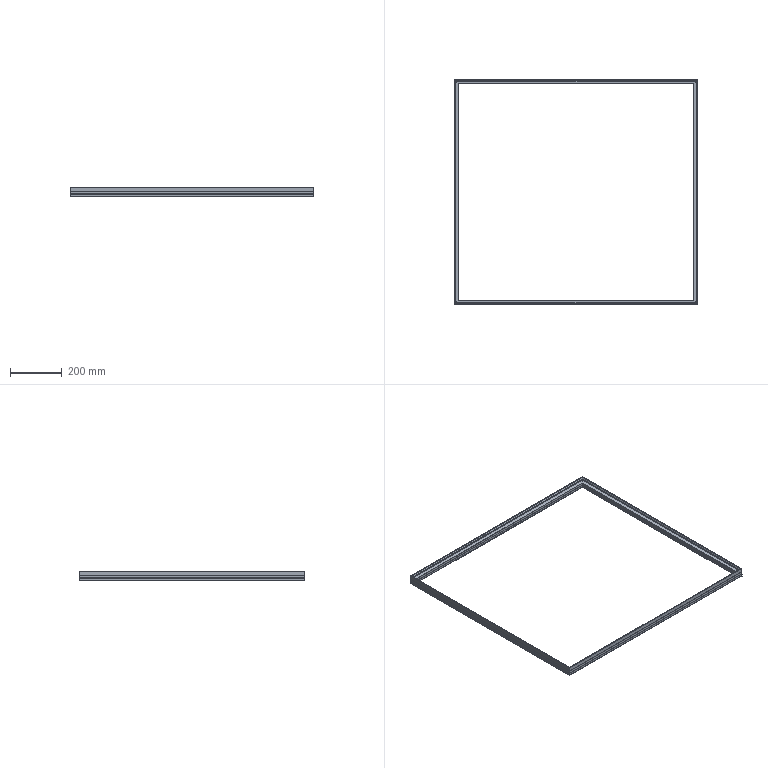Part | 4 solids | 96 faces | box 940 x 870 x 35 mm | volume 338218 mm3 | plane 96